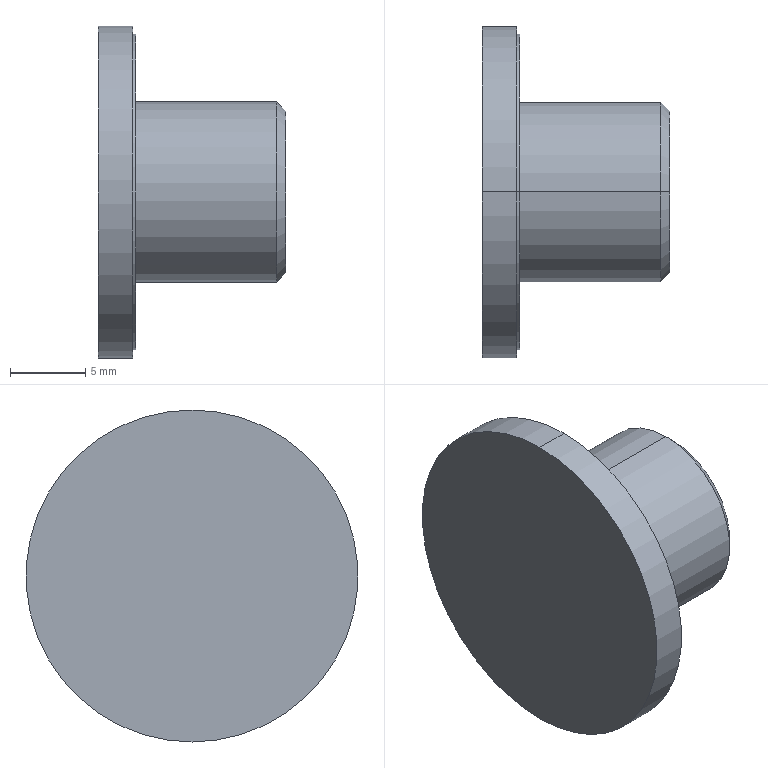Part | SolidWorks | features BaseBody 1 | 1 solid | 43 faces | box 12.5 x 22.1 x 22.1 mm | volume 1625 mm3 | cylinder 17 | plane 16 | cone 10 | commonest cylinder face diameters 1 x8 8.3 x2 12 x2 21 x2 22.1 x2 1.2 x1
STEP:
#1=CARTESIAN_POINT('',(49.5,0.,-11.05));
#2=VERTEX_POINT('',#1);
#3=CARTESIAN_POINT('',(49.5,0.,11.05));
#4=VERTEX_POINT('',#3);
#5=CARTESIAN_POINT('',(49.5,0.,0.));
#6=DIRECTION('',(1.,0.,0.));
#7=DIRECTION('',(0.,0.,-1.));
#8=AXIS2_PLACEMENT_3D('',#5,#6,#7);
#9=CIRCLE('',#8,11.05);
#10=EDGE_CURVE('',#2,#4,#9,.T.);
#11=ORIENTED_EDGE('',*,*,#10,.T.);
#12=CARTESIAN_POINT('',(51.8,0.,11.05));
#13=VERTEX_POINT('',#12);
#14=CARTESIAN_POINT('',(52.,0.,11.05));
#15=DIRECTION('',(1.,0.,0.));
#16=VECTOR('',#15,1000.);
#17=LINE('',#14,#16);
#18=EDGE_CURVE('',#4,#13,#17,.T.);
#19=ORIENTED_EDGE('',*,*,#18,.T.);
#20=CARTESIAN_POINT('',(51.8,0.,-11.05));
#21=VERTEX_POINT('',#20);
#22=CARTESIAN_POINT('',(51.8,0.,0.));
#23=DIRECTION('',(-1.,0.,0.));
#24=DIRECTION('',(0.,0.,-1.));
#25=AXIS2_PLACEMENT_3D('',#22,#23,#24);
#26=CIRCLE('',#25,11.05);
#27=EDGE_CURVE('',#13,#21,#26,.T.);
#28=ORIENTED_EDGE('',*,*,#27,.T.);
#29=CARTESIAN_POINT('',(52.,0.,-11.05));
#30=DIRECTION('',(1.,0.,0.));
#31=VECTOR('',#30,1000.);
#32=LINE('',#29,#31);
#33=EDGE_CURVE('',#2,#21,#32,.T.);
#34=ORIENTED_EDGE('',*,*,#33,.F.);
#35=EDGE_LOOP('',(#11,#19,#28,#34));
#36=FACE_OUTER_BOUND('',#35,.T.);
#37=CARTESIAN_POINT('',(52.,0.,0.));
#38=DIRECTION('',(1.,0.,0.));
#39=DIRECTION('',(0.,0.,-1.));
#40=AXIS2_PLACEMENT_3D('',#37,#38,#39);
#41=CYLINDRICAL_SURFACE('',#40,11.05);
#42=ADVANCED_FACE('',(#36),#41,.T.);
#43=CARTESIAN_POINT('',(51.8,0.,10.5));
#44=VERTEX_POINT('',#43);
#45=CARTESIAN_POINT('',(51.8,0.,-10.5));
#46=VERTEX_POINT('',#45);
#47=CARTESIAN_POINT('',(51.8,0.,0.));
#48=DIRECTION('',(-1.,0.,0.));
#49=DIRECTION('',(0.,0.,-1.));
#50=AXIS2_PLACEMENT_3D('',#47,#48,#49);
#51=CIRCLE('',#50,10.5);
#52=EDGE_CURVE('',#44,#46,#51,.T.);
#53=ORIENTED_EDGE('',*,*,#52,.F.);
#54=CARTESIAN_POINT('',(52.,0.,10.5));
#55=VERTEX_POINT('',#54);
#56=CARTESIAN_POINT('',(52.,0.,10.5));
#57=DIRECTION('',(1.,0.,0.));
#58=VECTOR('',#57,1000.);
#59=LINE('',#56,#58);
#60=EDGE_CURVE('',#44,#55,#59,.T.);
#61=ORIENTED_EDGE('',*,*,#60,.T.);
#62=CARTESIAN_POINT('',(52.,0.,-10.5));
#63=VERTEX_POINT('',#62);
#64=CARTESIAN_POINT('',(52.,0.,0.));
#65=DIRECTION('',(-1.,0.,0.));
#66=DIRECTION('',(0.,0.,-1.));
#67=AXIS2_PLACEMENT_3D('',#64,#65,#66);
#68=CIRCLE('',#67,10.5);
#69=EDGE_CURVE('',#55,#63,#68,.T.);
#70=ORIENTED_EDGE('',*,*,#69,.T.);
#71=CARTESIAN_POINT('',(52.,0.,-10.5));
#72=DIRECTION('',(1.,0.,0.));
#73=VECTOR('',#72,1000.);
#74=LINE('',#71,#73);
#75=EDGE_CURVE('',#46,#63,#74,.T.);
#76=ORIENTED_EDGE('',*,*,#75,.F.);
#77=EDGE_LOOP('',(#53,#61,#70,#76));
#78=FACE_OUTER_BOUND('',#77,.T.);
#79=CARTESIAN_POINT('',(52.,0.,0.));
#80=DIRECTION('',(1.,0.,0.));
#81=DIRECTION('',(0.,0.,-1.));
#82=AXIS2_PLACEMENT_3D('',#79,#80,#81);
#83=CYLINDRICAL_SURFACE('',#82,10.5);
#84=ADVANCED_FACE('',(#78),#83,.T.);
#85=CARTESIAN_POINT('',(52.,0.,6.));
#86=VERTEX_POINT('',#85);
#87=CARTESIAN_POINT('',(52.,0.,-6.));
#88=VERTEX_POINT('',#87);
#89=CARTESIAN_POINT('',(52.,0.,0.));
#90=DIRECTION('',(-1.,0.,0.));
#91=DIRECTION('',(0.,0.,-1.));
#92=AXIS2_PLACEMENT_3D('',#89,#90,#91);
#93=CIRCLE('',#92,6.);
#94=EDGE_CURVE('',#86,#88,#93,.T.);
#95=ORIENTED_EDGE('',*,*,#94,.F.);
#96=CARTESIAN_POINT('',(61.386,0.,6.));
#97=VERTEX_POINT('',#96);
#98=CARTESIAN_POINT('',(56.693,0.,6.));
#99=DIRECTION('',(1.,0.,0.));
#100=VECTOR('',#99,1000.);
#101=LINE('',#98,#100);
#102=EDGE_CURVE('',#86,#97,#101,.T.);
#103=ORIENTED_EDGE('',*,*,#102,.T.);
#104=CARTESIAN_POINT('',(61.386,0.,-6.));
#105=VERTEX_POINT('',#104);
#106=CARTESIAN_POINT('',(61.386,0.,0.));
#107=DIRECTION('',(-1.,0.,0.));
#108=DIRECTION('',(0.,0.,-1.));
#109=AXIS2_PLACEMENT_3D('',#106,#107,#108);
#110=CIRCLE('',#109,6.);
#111=EDGE_CURVE('',#97,#105,#110,.T.);
#112=ORIENTED_EDGE('',*,*,#111,.T.);
#113=CARTESIAN_POINT('',(56.693,0.,-6.));
#114=DIRECTION('',(1.,0.,0.));
#115=VECTOR('',#114,1000.);
#116=LINE('',#113,#115);
#117=EDGE_CURVE('',#88,#105,#116,.T.);
#118=ORIENTED_EDGE('',*,*,#117,.F.);
#119=EDGE_LOOP('',(#95,#103,#112,#118));
#120=FACE_OUTER_BOUND('',#119,.T.);
#121=CARTESIAN_POINT('',(56.693,0.,0.));
#122=DIRECTION('',(1.,0.,0.));
#123=DIRECTION('',(0.,0.,-1.));
#124=AXIS2_PLACEMENT_3D('',#121,#122,#123);
#125=CYLINDRICAL_SURFACE('',#124,6.);
#126=ADVANCED_FACE('',(#120),#125,.T.);
#127=CARTESIAN_POINT('',(62.,0.,5.387));
#128=VERTEX_POINT('',#127);
#129=CARTESIAN_POINT('',(62.,0.,-5.387));
#130=VERTEX_POINT('',#129);
#131=CARTESIAN_POINT('',(62.,0.,0.));
#132=DIRECTION('',(-1.,0.,0.));
#133=DIRECTION('',(0.,0.,1.));
#134=AXIS2_PLACEMENT_3D('',#131,#132,#133);
#135=CIRCLE('',#134,5.387);
#136=EDGE_CURVE('',#128,#130,#135,.T.);
#137=ORIENTED_EDGE('',*,*,#136,.T.);
#138=CARTESIAN_POINT('',(61.387,0.,-6.));
#139=DIRECTION('',(-0.7071,0.,-0.7071));
#140=VECTOR('',#139,1000.);
#141=LINE('',#138,#140);
#142=EDGE_CURVE('',#130,#105,#141,.T.);
#143=ORIENTED_EDGE('',*,*,#142,.T.);
#144=ORIENTED_EDGE('',*,*,#111,.F.);
#145=CARTESIAN_POINT('',(61.387,0.,6.));
#146=DIRECTION('',(-0.7071,0.,0.7071));
#147=VECTOR('',#146,1000.);
#148=LINE('',#145,#147);
#149=EDGE_CURVE('',#128,#97,#148,.T.);
#150=ORIENTED_EDGE('',*,*,#149,.F.);
#151=EDGE_LOOP('',(#137,#143,#144,#150));
#152=FACE_OUTER_BOUND('',#151,.T.);
#153=CARTESIAN_POINT('',(61.387,0.,0.));
#154=DIRECTION('',(-1.,0.,0.));
#155=DIRECTION('',(0.,0.,1.));
#156=AXIS2_PLACEMENT_3D('',#153,#154,#155);
#157=CONICAL_SURFACE('',#156,6.,0.7854);
#158=ADVANCED_FACE('',(#152),#157,.T.);
#159=CARTESIAN_POINT('',(53.1,0.,4.15));
#160=VERTEX_POINT('',#159);
#161=CARTESIAN_POINT('',(53.1,0.,-4.15));
#162=VERTEX_POINT('',#161);
#163=CARTESIAN_POINT('',(53.1,0.,0.));
#164=DIRECTION('',(1.,0.,0.));
#165=DIRECTION('',(0.,0.,-1.));
#166=AXIS2_PLACEMENT_3D('',#163,#164,#165);
#167=CIRCLE('',#166,4.15);
#168=EDGE_CURVE('',#160,#162,#167,.T.);
#169=ORIENTED_EDGE('',*,*,#168,.F.);
#170=CARTESIAN_POINT('',(62.,0.,4.15));
#171=VERTEX_POINT('',#170);
#172=CARTESIAN_POINT('',(57.55,0.,4.15));
#173=DIRECTION('',(1.,0.,0.));
#174=VECTOR('',#173,1000.);
#175=LINE('',#172,#174);
#176=EDGE_CURVE('',#160,#171,#175,.T.);
#177=ORIENTED_EDGE('',*,*,#176,.T.);
#178=CARTESIAN_POINT('',(62.,0.,-4.15));
#179=VERTEX_POINT('',#178);
#180=CARTESIAN_POINT('',(62.,0.,0.));
#181=DIRECTION('',(-1.,0.,0.));
#182=DIRECTION('',(0.,0.,-1.));
#183=AXIS2_PLACEMENT_3D('',#180,#181,#182);
#184=CIRCLE('',#183,4.15);
#185=EDGE_CURVE('',#179,#171,#184,.T.);
#186=ORIENTED_EDGE('',*,*,#185,.F.);
#187=CARTESIAN_POINT('',(57.55,0.,-4.15));
#188=DIRECTION('',(1.,0.,0.));
#189=VECTOR('',#188,1000.);
#190=LINE('',#187,#189);
#191=EDGE_CURVE('',#162,#179,#190,.T.);
#192=ORIENTED_EDGE('',*,*,#191,.F.);
#193=EDGE_LOOP('',(#169,#177,#186,#192));
#194=FACE_OUTER_BOUND('',#193,.T.);
#195=CARTESIAN_POINT('',(57.55,0.,0.));
#196=DIRECTION('',(1.,0.,0.));
#197=DIRECTION('',(0.,0.,-1.));
#198=AXIS2_PLACEMENT_3D('',#195,#196,#197);
#199=CYLINDRICAL_SURFACE('',#198,4.15);
#200=ADVANCED_FACE('',(#194),#199,.F.);
#201=CARTESIAN_POINT('',(53.1,0.,3.));
#202=VERTEX_POINT('',#201);
#203=CARTESIAN_POINT('',(53.1,0.,2.));
#204=VERTEX_POINT('',#203);
#205=CARTESIAN_POINT('',(53.1,0.,2.5));
#206=DIRECTION('',(-1.,0.,0.));
#207=DIRECTION('',(0.,0.,-1.));
#208=AXIS2_PLACEMENT_3D('',#205,#206,#207);
#209=CIRCLE('',#208,0.5);
#210=EDGE_CURVE('',#202,#204,#209,.T.);
#211=ORIENTED_EDGE('',*,*,#210,.F.);
#212=CARTESIAN_POINT('',(59.067,0.,3.));
#213=VERTEX_POINT('',#212);
#214=CARTESIAN_POINT('',(56.083,0.,3.));
#215=DIRECTION('',(1.,0.,0.));
#216=VECTOR('',#215,1000.);
#217=LINE('',#214,#216);
#218=EDGE_CURVE('',#202,#213,#217,.T.);
#219=ORIENTED_EDGE('',*,*,#218,.T.);
#220=CARTESIAN_POINT('',(59.067,0.5,2.5));
#221=VERTEX_POINT('',#220);
#222=CARTESIAN_POINT('',(59.067,0.,2.5));
#223=DIRECTION('',(-1.,0.,0.));
#224=DIRECTION('',(0.,0.,-1.));
#225=AXIS2_PLACEMENT_3D('',#222,#223,#224);
#226=CIRCLE('',#225,0.5);
#227=EDGE_CURVE('',#213,#221,#226,.T.);
#228=ORIENTED_EDGE('',*,*,#227,.T.);
#229=CARTESIAN_POINT('',(59.067,0.,2.));
#230=VERTEX_POINT('',#229);
#231=CARTESIAN_POINT('',(59.067,0.,2.5));
#232=DIRECTION('',(-1.,0.,0.));
#233=DIRECTION('',(0.,0.,-1.));
#234=AXIS2_PLACEMENT_3D('',#231,#232,#233);
#235=CIRCLE('',#234,0.5);
#236=EDGE_CURVE('',#221,#230,#235,.T.);
#237=ORIENTED_EDGE('',*,*,#236,.T.);
#238=CARTESIAN_POINT('',(56.083,0.,2.));
#239=DIRECTION('',(1.,0.,0.));
#240=VECTOR('',#239,1000.);
#241=LINE('',#238,#240);
#242=EDGE_CURVE('',#204,#230,#241,.T.);
#243=ORIENTED_EDGE('',*,*,#242,.F.);
#244=EDGE_LOOP('',(#211,#219,#228,#237,#243));
#245=FACE_OUTER_BOUND('',#244,.T.);
#246=CARTESIAN_POINT('',(56.083,0.,2.5));
#247=DIRECTION('',(1.,0.,0.));
#248=DIRECTION('',(0.,0.,-1.));
#249=AXIS2_PLACEMENT_3D('',#246,#247,#248);
#250=CYLINDRICAL_SURFACE('',#249,0.5);
#251=ADVANCED_FACE('',(#245),#250,.T.);
#252=CARTESIAN_POINT('',(53.1,-2.5,0.5));
#253=VERTEX_POINT('',#252);
#254=CARTESIAN_POINT('',(53.1,-2.5,-0.5));
#255=VERTEX_POINT('',#254);
#256=CARTESIAN_POINT('',(53.1,-2.5,0.));
#257=DIRECTION('',(-1.,0.,0.));
#258=DIRECTION('',(0.,0.,-1.));
#259=AXIS2_PLACEMENT_3D('',#256,#257,#258);
#260=CIRCLE('',#259,0.5);
#261=EDGE_CURVE('',#253,#255,#260,.T.);
#262=ORIENTED_EDGE('',*,*,#261,.F.);
#263=CARTESIAN_POINT('',(59.067,-2.5,0.5));
#264=VERTEX_POINT('',#263);
#265=CARTESIAN_POINT('',(56.083,-2.5,0.5));
#266=DIRECTION('',(1.,0.,0.));
#267=VECTOR('',#266,1000.);
#268=LINE('',#265,#267);
#269=EDGE_CURVE('',#253,#264,#268,.T.);
#270=ORIENTED_EDGE('',*,*,#269,.T.);
#271=CARTESIAN_POINT('',(59.067,-2.5,-0.5));
#272=VERTEX_POINT('',#271);
#273=CARTESIAN_POINT('',(59.067,-2.5,0.));
#274=DIRECTION('',(-1.,0.,0.));
#275=DIRECTION('',(0.,0.,-1.));
#276=AXIS2_PLACEMENT_3D('',#273,#274,#275);
#277=CIRCLE('',#276,0.5);
#278=EDGE_CURVE('',#264,#272,#277,.T.);
#279=ORIENTED_EDGE('',*,*,#278,.T.);
#280=CARTESIAN_POINT('',(56.083,-2.5,-0.5));
#281=DIRECTION('',(1.,0.,0.));
#282=VECTOR('',#281,1000.);
#283=LINE('',#280,#282);
#284=EDGE_CURVE('',#255,#272,#283,.T.);
#285=ORIENTED_EDGE('',*,*,#284,.F.);
#286=EDGE_LOOP('',(#262,#270,#279,#285));
#287=FACE_OUTER_BOUND('',#286,.T.);
#288=CARTESIAN_POINT('',(56.083,-2.5,0.));
#289=DIRECTION('',(1.,0.,0.));
#290=DIRECTION('',(0.,0.,-1.));
#291=AXIS2_PLACEMENT_3D('',#288,#289,#290);
#292=CYLINDRICAL_SURFACE('',#291,0.5);
#293=ADVANCED_FACE('',(#287),#292,.T.);
#294=CARTESIAN_POINT('',(53.1,0.,-2.));
#295=VERTEX_POINT('',#294);
#296=CARTESIAN_POINT('',(53.1,0.,-3.));
#297=VERTEX_POINT('',#296);
#298=CARTESIAN_POINT('',(53.1,0.,-2.5));
#299=DIRECTION('',(-1.,0.,0.));
#300=DIRECTION('',(0.,0.,-1.));
#301=AXIS2_PLACEMENT_3D('',#298,#299,#300);
#302=CIRCLE('',#301,0.5);
#303=EDGE_CURVE('',#295,#297,#302,.T.);
#304=ORIENTED_EDGE('',*,*,#303,.F.);
#305=CARTESIAN_POINT('',(59.067,0.,-2.));
#306=VERTEX_POINT('',#305);
#307=CARTESIAN_POINT('',(56.083,0.,-2.));
#308=DIRECTION('',(1.,0.,0.));
#309=VECTOR('',#308,1000.);
#310=LINE('',#307,#309);
#311=EDGE_CURVE('',#295,#306,#310,.T.);
#312=ORIENTED_EDGE('',*,*,#311,.T.);
#313=CARTESIAN_POINT('',(59.067,0.5,-2.5));
#314=VERTEX_POINT('',#313);
#315=CARTESIAN_POINT('',(59.067,0.,-2.5));
#316=DIRECTION('',(-1.,0.,0.));
#317=DIRECTION('',(0.,0.,-1.));
#318=AXIS2_PLACEMENT_3D('',#315,#316,#317);
#319=CIRCLE('',#318,0.5);
#320=EDGE_CURVE('',#306,#314,#319,.T.);
#321=ORIENTED_EDGE('',*,*,#320,.T.);
#322=CARTESIAN_POINT('',(59.067,0.,-3.));
#323=VERTEX_POINT('',#322);
#324=CARTESIAN_POINT('',(59.067,0.,-2.5));
#325=DIRECTION('',(-1.,0.,0.));
#326=DIRECTION('',(0.,0.,-1.));
#327=AXIS2_PLACEMENT_3D('',#324,#325,#326);
#328=CIRCLE('',#327,0.5);
#329=EDGE_CURVE('',#314,#323,#328,.T.);
#330=ORIENTED_EDGE('',*,*,#329,.T.);
#331=CARTESIAN_POINT('',(56.083,0.,-3.));
#332=DIRECTION('',(1.,0.,0.));
#333=VECTOR('',#332,1000.);
#334=LINE('',#331,#333);
#335=EDGE_CURVE('',#297,#323,#334,.T.);
#336=ORIENTED_EDGE('',*,*,#335,.F.);
#337=EDGE_LOOP('',(#304,#312,#321,#330,#336));
#338=FACE_OUTER_BOUND('',#337,.T.);
#339=CARTESIAN_POINT('',(56.083,0.,-2.5));
#340=DIRECTION('',(1.,0.,0.));
#341=DIRECTION('',(0.,0.,-1.));
#342=AXIS2_PLACEMENT_3D('',#339,#340,#341);
#343=CYLINDRICAL_SURFACE('',#342,0.5);
#344=ADVANCED_FACE('',(#338),#343,.T.);
#345=CARTESIAN_POINT('',(53.1,2.5,0.5));
#346=VERTEX_POINT('',#345);
#347=CARTESIAN_POINT('',(53.1,2.5,-0.5));
#348=VERTEX_POINT('',#347);
#349=CARTESIAN_POINT('',(53.1,2.5,0.));
#350=DIRECTION('',(-1.,0.,0.));
#351=DIRECTION('',(0.,0.,-1.));
#352=AXIS2_PLACEMENT_3D('',#349,#350,#351);
#353=CIRCLE('',#352,0.5);
#354=EDGE_CURVE('',#346,#348,#353,.T.);
#355=ORIENTED_EDGE('',*,*,#354,.F.);
#356=CARTESIAN_POINT('',(59.067,2.5,0.5));
#357=VERTEX_POINT('',#356);
#358=CARTESIAN_POINT('',(56.083,2.5,0.5));
#359=DIRECTION('',(1.,0.,0.));
#360=VECTOR('',#359,1000.);
#361=LINE('',#358,#360);
#362=EDGE_CURVE('',#346,#357,#361,.T.);
#363=ORIENTED_EDGE('',*,*,#362,.T.);
#364=CARTESIAN_POINT('',(59.067,2.5,-0.5));
#365=VERTEX_POINT('',#364);
#366=CARTESIAN_POINT('',(59.067,2.5,0.));
#367=DIRECTION('',(-1.,0.,0.));
#368=DIRECTION('',(0.,0.,-1.));
#369=AXIS2_PLACEMENT_3D('',#366,#367,#368);
#370=CIRCLE('',#369,0.5);
#371=EDGE_CURVE('',#357,#365,#370,.T.);
#372=ORIENTED_EDGE('',*,*,#371,.T.);
#373=CARTESIAN_POINT('',(56.083,2.5,-0.5));
#374=DIRECTION('',(1.,0.,0.));
#375=VECTOR('',#374,1000.);
#376=LINE('',#373,#375);
#377=EDGE_CURVE('',#348,#365,#376,.T.);
#378=ORIENTED_EDGE('',*,*,#377,.F.);
#379=EDGE_LOOP('',(#355,#363,#372,#378));
#380=FACE_OUTER_BOUND('',#379,.T.);
#381=CARTESIAN_POINT('',(56.083,2.5,0.));
#382=DIRECTION('',(1.,0.,0.));
#383=DIRECTION('',(0.,0.,-1.));
#384=AXIS2_PLACEMENT_3D('',#381,#382,#383);
#385=CYLINDRICAL_SURFACE('',#384,0.5);
#386=ADVANCED_FACE('',(#380),#385,.T.);
#387=CARTESIAN_POINT('',(60.,-0.25,2.5));
#388=VERTEX_POINT('',#387);
#389=CARTESIAN_POINT('',(60.,0.25,2.5));
#390=VERTEX_POINT('',#389);
#391=CARTESIAN_POINT('',(60.,0.,2.5));
#392=DIRECTION('',(-1.,0.,0.));
#393=DIRECTION('',(0.,-1.,0.));
#394=AXIS2_PLACEMENT_3D('',#391,#392,#393);
#395=CIRCLE('',#394,0.25);
#396=EDGE_CURVE('',#388,#390,#395,.T.);
#397=ORIENTED_EDGE('',*,*,#396,.T.);
#398=CARTESIAN_POINT('',(59.067,0.5,2.5));
#399=DIRECTION('',(-0.9659,0.2588,0.));
#400=VECTOR('',#399,1000.);
#401=LINE('',#398,#400);
#402=EDGE_CURVE('',#390,#221,#401,.T.);
#403=ORIENTED_EDGE('',*,*,#402,.T.);
#404=ORIENTED_EDGE('',*,*,#227,.F.);
#405=CARTESIAN_POINT('',(59.067,-0.5,2.5));
#406=VERTEX_POINT('',#405);
#407=CARTESIAN_POINT('',(59.067,0.,2.5));
#408=DIRECTION('',(-1.,0.,0.));
#409=DIRECTION('',(0.,0.,-1.));
#410=AXIS2_PLACEMENT_3D('',#407,#408,#409);
#411=CIRCLE('',#410,0.5);
#412=EDGE_CURVE('',#406,#213,#411,.T.);
#413=ORIENTED_EDGE('',*,*,#412,.F.);
#414=CARTESIAN_POINT('',(59.067,-0.5,2.5));
#415=DIRECTION('',(-0.9659,-0.2588,0.));
#416=VECTOR('',#415,1000.);
#417=LINE('',#414,#416);
#418=EDGE_CURVE('',#388,#406,#417,.T.);
#419=ORIENTED_EDGE('',*,*,#418,.F.);
#420=EDGE_LOOP('',(#397,#403,#404,#413,#419));
#421=FACE_OUTER_BOUND('',#420,.T.);
#422=CARTESIAN_POINT('',(59.067,0.,2.5));
#423=DIRECTION('',(-1.,0.,0.));
#424=DIRECTION('',(0.,-1.,0.));
#425=AXIS2_PLACEMENT_3D('',#422,#423,#424);
#426=CONICAL_SURFACE('',#425,0.5,0.2618);
#427=ADVANCED_FACE('',(#421),#426,.T.);
#428=CARTESIAN_POINT('',(60.,-2.5,0.25));
#429=VERTEX_POINT('',#428);
#430=CARTESIAN_POINT('',(60.,-2.5,-0.25));
#431=VERTEX_POINT('',#430);
#432=CARTESIAN_POINT('',(60.,-2.5,0.));
#433=DIRECTION('',(-1.,0.,0.));
#434=DIRECTION('',(0.,0.,1.));
#435=AXIS2_PLACEMENT_3D('',#432,#433,#434);
#436=CIRCLE('',#435,0.25);
#437=EDGE_CURVE('',#429,#431,#436,.T.);
#438=ORIENTED_EDGE('',*,*,#437,.T.);
#439=CARTESIAN_POINT('',(59.067,-2.5,-0.5));
#440=DIRECTION('',(-0.9659,0.,-0.2588));
#441=VECTOR('',#440,1000.);
#442=LINE('',#439,#441);
#443=EDGE_CURVE('',#431,#272,#442,.T.);
#444=ORIENTED_EDGE('',*,*,#443,.T.);
#445=ORIENTED_EDGE('',*,*,#278,.F.);
#446=CARTESIAN_POINT('',(59.067,-2.5,0.5));
#447=DIRECTION('',(-0.9659,0.,0.2588));
#448=VECTOR('',#447,1000.);
#449=LINE('',#446,#448);
#450=EDGE_CURVE('',#429,#264,#449,.T.);
#451=ORIENTED_EDGE('',*,*,#450,.F.);
#452=EDGE_LOOP('',(#438,#444,#445,#451));
#453=FACE_OUTER_BOUND('',#452,.T.);
#454=CARTESIAN_POINT('',(59.067,-2.5,0.));
#455=DIRECTION('',(-1.,0.,0.));
#456=DIRECTION('',(0.,0.,1.));
#457=AXIS2_PLACEMENT_3D('',#454,#455,#456);
#458=CONICAL_SURFACE('',#457,0.5,0.2618);
#459=ADVANCED_FACE('',(#453),#458,.T.);
#460=CARTESIAN_POINT('',(60.,-0.25,-2.5));
#461=VERTEX_POINT('',#460);
#462=CARTESIAN_POINT('',(60.,0.25,-2.5));
#463=VERTEX_POINT('',#462);
#464=CARTESIAN_POINT('',(60.,0.,-2.5));
#465=DIRECTION('',(-1.,0.,0.));
#466=DIRECTION('',(0.,-1.,0.));
#467=AXIS2_PLACEMENT_3D('',#464,#465,#466);
#468=CIRCLE('',#467,0.25);
#469=EDGE_CURVE('',#461,#463,#468,.T.);
#470=ORIENTED_EDGE('',*,*,#469,.T.);
#471=CARTESIAN_POINT('',(59.067,0.5,-2.5));
#472=DIRECTION('',(-0.9659,0.2588,0.));
#473=VECTOR('',#472,1000.);
#474=LINE('',#471,#473);
#475=EDGE_CURVE('',#463,#314,#474,.T.);
#476=ORIENTED_EDGE('',*,*,#475,.T.);
#477=ORIENTED_EDGE('',*,*,#320,.F.);
#478=CARTESIAN_POINT('',(59.067,-0.5,-2.5));
#479=VERTEX_POINT('',#478);
#480=CARTESIAN_POINT('',(59.067,0.,-2.5));
#481=DIRECTION('',(-1.,0.,0.));
#482=DIRECTION('',(0.,0.,-1.));
#483=AXIS2_PLACEMENT_3D('',#480,#481,#482);
#484=CIRCLE('',#483,0.5);
#485=EDGE_CURVE('',#479,#306,#484,.T.);
#486=ORIENTED_EDGE('',*,*,#485,.F.);
#487=CARTESIAN_POINT('',(59.067,-0.5,-2.5));
#488=DIRECTION('',(-0.9659,-0.2588,0.));
#489=VECTOR('',#488,1000.);
#490=LINE('',#487,#489);
#491=EDGE_CURVE('',#461,#479,#490,.T.);
#492=ORIENTED_EDGE('',*,*,#491,.F.);
#493=EDGE_LOOP('',(#470,#476,#477,#486,#492));
#494=FACE_OUTER_BOUND('',#493,.T.);
#495=CARTESIAN_POINT('',(59.067,0.,-2.5));
#496=DIRECTION('',(-1.,0.,0.));
#497=DIRECTION('',(0.,-1.,0.));
#498=AXIS2_PLACEMENT_3D('',#495,#496,#497);
#499=CONICAL_SURFACE('',#498,0.5,0.2618);
#500=ADVANCED_FACE('',(#494),#499,.T.);
#501=CARTESIAN_POINT('',(60.,2.5,0.25));
#502=VERTEX_POINT('',#501);
#503=CARTESIAN_POINT('',(60.,2.5,-0.25));
#504=VERTEX_POINT('',#503);
#505=CARTESIAN_POINT('',(60.,2.5,0.));
#506=DIRECTION('',(-1.,0.,0.));
#507=DIRECTION('',(0.,0.,1.));
#508=AXIS2_PLACEMENT_3D('',#505,#506,#507);
#509=CIRCLE('',#508,0.25);
#510=EDGE_CURVE('',#502,#504,#509,.T.);
#511=ORIENTED_EDGE('',*,*,#510,.T.);
#512=CARTESIAN_POINT('',(59.067,2.5,-0.5));
#513=DIRECTION('',(-0.9659,0.,-0.2588));
#514=VECTOR('',#513,1000.);
#515=LINE('',#512,#514);
#516=EDGE_CURVE('',#504,#365,#515,.T.);
#517=ORIENTED_EDGE('',*,*,#516,.T.);
#518=ORIENTED_EDGE('',*,*,#371,.F.);
#519=CARTESIAN_POINT('',(59.067,2.5,0.5));
#520=DIRECTION('',(-0.9659,0.,0.2588));
#521=VECTOR('',#520,1000.);
#522=LINE('',#519,#521);
#523=EDGE_CURVE('',#502,#357,#522,.T.);
#524=ORIENTED_EDGE('',*,*,#523,.F.);
#525=EDGE_LOOP('',(#511,#517,#518,#524));
#526=FACE_OUTER_BOUND('',#525,.T.);
#527=CARTESIAN_POINT('',(59.067,2.5,0.));
#528=DIRECTION('',(-1.,0.,0.));
#529=DIRECTION('',(0.,0.,1.));
#530=AXIS2_PLACEMENT_3D('',#527,#528,#529);
#531=CONICAL_SURFACE('',#530,0.5,0.2618);
#532=ADVANCED_FACE('',(#526),#531,.T.);
#533=ORIENTED_EDGE('',*,*,#10,.F.);
#534=CARTESIAN_POINT('',(49.5,0.,0.));
#535=DIRECTION('',(1.,0.,0.));
#536=DIRECTION('',(0.,0.,-1.));
#537=AXIS2_PLACEMENT_3D('',#534,#535,#536);
#538=CIRCLE('',#537,11.05);
#539=EDGE_CURVE('',#4,#2,#538,.T.);
#540=ORIENTED_EDGE('',*,*,#539,.F.);
#541=EDGE_LOOP('',(#533,#540));
#542=FACE_OUTER_BOUND('',#541,.T.);
#543=CARTESIAN_POINT('',(49.5,0.,0.));
#544=DIRECTION('',(1.,0.,0.));
#545=DIRECTION('',(0.,0.,-1.));
#546=AXIS2_PLACEMENT_3D('',#543,#544,#545);
#547=PLANE('',#546);
#548=ADVANCED_FACE('',(#542),#547,.F.);
#549=ORIENTED_EDGE('',*,*,#18,.F.);
#550=ORIENTED_EDGE('',*,*,#539,.T.);
#551=ORIENTED_EDGE('',*,*,#33,.T.);
#552=CARTESIAN_POINT('',(51.8,0.,0.));
#553=DIRECTION('',(-1.,0.,0.));
#554=DIRECTION('',(0.,0.,-1.));
#555=AXIS2_PLACEMENT_3D('',#552,#553,#554);
#556=CIRCLE('',#555,11.05);
#557=EDGE_CURVE('',#21,#13,#556,.T.);
#558=ORIENTED_EDGE('',*,*,#557,.T.);
#559=EDGE_LOOP('',(#549,#550,#551,#558));
#560=FACE_OUTER_BOUND('',#559,.T.);
#561=CARTESIAN_POINT('',(52.,0.,0.));
#562=DIRECTION('',(1.,0.,0.));
#563=DIRECTION('',(0.,0.,-1.));
#564=AXIS2_PLACEMENT_3D('',#561,#562,#563);
#565=CYLINDRICAL_SURFACE('',#564,11.05);
#566=ADVANCED_FACE('',(#560),#565,.T.);
#567=CARTESIAN_POINT('',(51.8,0.,0.));
#568=DIRECTION('',(-1.,0.,0.));
#569=DIRECTION('',(0.,0.,-1.));
#570=AXIS2_PLACEMENT_3D('',#567,#568,#569);
#571=CIRCLE('',#570,10.5);
#572=EDGE_CURVE('',#46,#44,#571,.T.);
#573=ORIENTED_EDGE('',*,*,#572,.T.);
#574=ORIENTED_EDGE('',*,*,#52,.T.);
#575=EDGE_LOOP('',(#573,#574));
#576=FACE_BOUND('',#575,.T.);
#577=ORIENTED_EDGE('',*,*,#557,.F.);
#578=ORIENTED_EDGE('',*,*,#27,.F.);
#579=EDGE_LOOP('',(#577,#578));
#580=FACE_OUTER_BOUND('',#579,.T.);
#581=CARTESIAN_POINT('',(51.8,0.,0.));
#582=DIRECTION('',(1.,0.,0.));
#583=DIRECTION('',(0.,0.,-1.));
#584=AXIS2_PLACEMENT_3D('',#581,#582,#583);
#585=PLANE('',#584);
#586=ADVANCED_FACE('',(#576,#580),#585,.T.);
#587=ORIENTED_EDGE('',*,*,#60,.F.);
#588=ORIENTED_EDGE('',*,*,#572,.F.);
#589=ORIENTED_EDGE('',*,*,#75,.T.);
#590=CARTESIAN_POINT('',(52.,0.,0.));
#591=DIRECTION('',(-1.,0.,0.));
#592=DIRECTION('',(0.,0.,-1.));
#593=AXIS2_PLACEMENT_3D('',#590,#591,#592);
#594=CIRCLE('',#593,10.5);
#595=EDGE_CURVE('',#63,#55,#594,.T.);
#596=ORIENTED_EDGE('',*,*,#595,.T.);
#597=EDGE_LOOP('',(#587,#588,#589,#596));
#598=FACE_OUTER_BOUND('',#597,.T.);
#599=CARTESIAN_POINT('',(52.,0.,0.));
#600=DIRECTION('',(1.,0.,0.));
#601=DIRECTION('',(0.,0.,-1.));
#602=AXIS2_PLACEMENT_3D('',#599,#600,#601);
#603=CYLINDRICAL_SURFACE('',#602,10.5);
#604=ADVANCED_FACE('',(#598),#603,.T.);
#605=CARTESIAN_POINT('',(52.,0.,0.));
#606=DIRECTION('',(-1.,0.,0.));
#607=DIRECTION('',(0.,0.,-1.));
#608=AXIS2_PLACEMENT_3D('',#605,#606,#607);
#609=CIRCLE('',#608,6.);
#610=EDGE_CURVE('',#88,#86,#609,.T.);
#611=ORIENTED_EDGE('',*,*,#610,.T.);
#612=ORIENTED_EDGE('',*,*,#94,.T.);
#613=EDGE_LOOP('',(#611,#612));
#614=FACE_BOUND('',#613,.T.);
#615=CARTESIAN_POINT('',(52.,6.35,0.7));
#616=VERTEX_POINT('',#615);
#617=CARTESIAN_POINT('',(52.,10.,0.));
#618=VERTEX_POINT('',#617);
#619=CARTESIAN_POINT('',(52.,6.35,0.7));
#620=DIRECTION('',(0.,0.9821,-0.1883));
#621=VECTOR('',#620,1000.);
#622=LINE('',#619,#621);
#623=EDGE_CURVE('',#616,#618,#622,.T.);
#624=ORIENTED_EDGE('',*,*,#623,.T.);
#625=CARTESIAN_POINT('',(52.,6.35,-0.7));
#626=VERTEX_POINT('',#625);
#627=CARTESIAN_POINT('',(52.,10.,0.));
#628=DIRECTION('',(0.,-0.9821,-0.1883));
#629=VECTOR('',#628,1000.);
#630=LINE('',#627,#629);
#631=EDGE_CURVE('',#618,#626,#630,.T.);
#632=ORIENTED_EDGE('',*,*,#631,.T.);
#633=CARTESIAN_POINT('',(52.,6.35,0.));
#634=DIRECTION('',(0.,0.,1.));
#635=VECTOR('',#634,1000.);
#636=LINE('',#633,#635);
#637=EDGE_CURVE('',#626,#616,#636,.T.);
#638=ORIENTED_EDGE('',*,*,#637,.T.);
#639=EDGE_LOOP('',(#624,#632,#638));
#640=FACE_BOUND('',#639,.T.);
#641=ORIENTED_EDGE('',*,*,#595,.F.);
#642=ORIENTED_EDGE('',*,*,#69,.F.);
#643=EDGE_LOOP('',(#641,#642));
#644=FACE_OUTER_BOUND('',#643,.T.);
#645=CARTESIAN_POINT('',(52.,0.,0.));
#646=DIRECTION('',(1.,0.,0.));
#647=DIRECTION('',(0.,0.,-1.));
#648=AXIS2_PLACEMENT_3D('',#645,#646,#647);
#649=PLANE('',#648);
#650=ADVANCED_FACE('',(#614,#640,#644),#649,.T.);
#651=ORIENTED_EDGE('',*,*,#102,.F.);
#652=ORIENTED_EDGE('',*,*,#610,.F.);
#653=ORIENTED_EDGE('',*,*,#117,.T.);
#654=CARTESIAN_POINT('',(61.386,0.,0.));
#655=DIRECTION('',(-1.,0.,0.));
#656=DIRECTION('',(0.,0.,-1.));
#657=AXIS2_PLACEMENT_3D('',#654,#655,#656);
#658=CIRCLE('',#657,6.);
#659=EDGE_CURVE('',#105,#97,#658,.T.);
#660=ORIENTED_EDGE('',*,*,#659,.T.);
#661=EDGE_LOOP('',(#651,#652,#653,#660));
#662=FACE_OUTER_BOUND('',#661,.T.);
#663=CARTESIAN_POINT('',(56.693,0.,0.));
#664=DIRECTION('',(1.,0.,0.));
#665=DIRECTION('',(0.,0.,-1.));
#666=AXIS2_PLACEMENT_3D('',#663,#664,#665);
#667=CYLINDRICAL_SURFACE('',#666,6.);
#668=ADVANCED_FACE('',(#662),#667,.T.);
#669=ORIENTED_EDGE('',*,*,#631,.F.);
#670=CARTESIAN_POINT('',(51.8,10.,0.));
#671=VERTEX_POINT('',#670);
#672=CARTESIAN_POINT('',(52.,10.,0.));
#673=DIRECTION('',(1.,0.,0.));
#674=VECTOR('',#673,1000.);
#675=LINE('',#672,#674);
#676=EDGE_CURVE('',#671,#618,#675,.T.);
#677=ORIENTED_EDGE('',*,*,#676,.F.);
#678=CARTESIAN_POINT('',(51.8,6.35,-0.7));
#679=VERTEX_POINT('',#678);
#680=CARTESIAN_POINT('',(51.8,6.35,-0.7));
#681=DIRECTION('',(0.,0.9821,0.1883));
#682=VECTOR('',#681,1000.);
#683=LINE('',#680,#682);
#684=EDGE_CURVE('',#679,#671,#683,.T.);
#685=ORIENTED_EDGE('',*,*,#684,.F.);
#686=CARTESIAN_POINT('',(52.,6.35,-0.7));
#687=DIRECTION('',(-1.,0.,0.));
#688=VECTOR('',#687,1000.);
#689=LINE('',#686,#688);
#690=EDGE_CURVE('',#626,#679,#689,.T.);
#691=ORIENTED_EDGE('',*,*,#690,.F.);
#692=EDGE_LOOP('',(#669,#677,#685,#691));
#693=FACE_OUTER_BOUND('',#692,.T.);
#694=CARTESIAN_POINT('',(52.,6.35,-0.7));
#695=DIRECTION('',(0.,0.1883,-0.9821));
#696=DIRECTION('',(0.,0.9821,0.1883));
#697=AXIS2_PLACEMENT_3D('',#694,#695,#696);
#698=PLANE('',#697);
#699=ADVANCED_FACE('',(#693),#698,.F.);
#700=ORIENTED_EDGE('',*,*,#623,.F.);
#701=CARTESIAN_POINT('',(51.8,6.35,0.7));
#702=VERTEX_POINT('',#701);
#703=CARTESIAN_POINT('',(52.,6.35,0.7));
#704=DIRECTION('',(1.,0.,0.));
#705=VECTOR('',#704,1000.);
#706=LINE('',#703,#705);
#707=EDGE_CURVE('',#702,#616,#706,.T.);
#708=ORIENTED_EDGE('',*,*,#707,.F.);
#709=CARTESIAN_POINT('',(51.8,10.,0.));
#710=DIRECTION('',(0.,-0.9821,0.1883));
#711=VECTOR('',#710,1000.);
#712=LINE('',#709,#711);
#713=EDGE_CURVE('',#671,#702,#712,.T.);
#714=ORIENTED_EDGE('',*,*,#713,.F.);
#715=ORIENTED_EDGE('',*,*,#676,.T.);
#716=EDGE_LOOP('',(#700,#708,#714,#715));
#717=FACE_OUTER_BOUND('',#716,.T.);
#718=CARTESIAN_POINT('',(52.,10.,0.));
#719=DIRECTION('',(0.,0.1883,0.9821));
#720=DIRECTION('',(0.,-0.9821,0.1883));
#721=AXIS2_PLACEMENT_3D('',#718,#719,#720);
#722=PLANE('',#721);
#723=ADVANCED_FACE('',(#717),#722,.F.);
#724=ORIENTED_EDGE('',*,*,#637,.F.);
#725=ORIENTED_EDGE('',*,*,#690,.T.);
#726=CARTESIAN_POINT('',(51.8,6.35,0.7));
#727=DIRECTION('',(0.,0.,-1.));
#728=VECTOR('',#727,1000.);
#729=LINE('',#726,#728);
#730=EDGE_CURVE('',#702,#679,#729,.T.);
#731=ORIENTED_EDGE('',*,*,#730,.F.);
#732=ORIENTED_EDGE('',*,*,#707,.T.);
#733=EDGE_LOOP('',(#724,#725,#731,#732));
#734=FACE_OUTER_BOUND('',#733,.T.);
#735=CARTESIAN_POINT('',(52.,6.35,0.7));
#736=DIRECTION('',(0.,-1.,0.));
#737=DIRECTION('',(0.,0.,-1.));
#738=AXIS2_PLACEMENT_3D('',#735,#736,#737);
#739=PLANE('',#738);
#740=ADVANCED_FACE('',(#734),#739,.F.);
#741=ORIENTED_EDGE('',*,*,#142,.F.);
#742=CARTESIAN_POINT('',(62.,0.,0.));
#743=DIRECTION('',(-1.,0.,0.));
#744=DIRECTION('',(0.,0.,1.));
#745=AXIS2_PLACEMENT_3D('',#742,#743,#744);
#746=CIRCLE('',#745,5.387);
#747=EDGE_CURVE('',#130,#128,#746,.T.);
#748=ORIENTED_EDGE('',*,*,#747,.T.);
#749=ORIENTED_EDGE('',*,*,#149,.T.);
#750=ORIENTED_EDGE('',*,*,#659,.F.);
#751=EDGE_LOOP('',(#741,#748,#749,#750));
#752=FACE_OUTER_BOUND('',#751,.T.);
#753=CARTESIAN_POINT('',(61.387,0.,0.));
#754=DIRECTION('',(-1.,0.,0.));
#755=DIRECTION('',(0.,0.,1.));
#756=AXIS2_PLACEMENT_3D('',#753,#754,#755);
#757=CONICAL_SURFACE('',#756,6.,0.7854);
#758=ADVANCED_FACE('',(#752),#757,.T.);
#759=ORIENTED_EDGE('',*,*,#730,.T.);
#760=ORIENTED_EDGE('',*,*,#684,.T.);
#761=ORIENTED_EDGE('',*,*,#713,.T.);
#762=EDGE_LOOP('',(#759,#760,#761));
#763=FACE_OUTER_BOUND('',#762,.T.);
#764=CARTESIAN_POINT('',(51.8,0.,0.));
#765=DIRECTION('',(1.,0.,0.));
#766=DIRECTION('',(0.,0.,-1.));
#767=AXIS2_PLACEMENT_3D('',#764,#765,#766);
#768=PLANE('',#767);
#769=ADVANCED_FACE('',(#763),#768,.T.);
#770=ORIENTED_EDGE('',*,*,#185,.T.);
#771=CARTESIAN_POINT('',(62.,0.,0.));
#772=DIRECTION('',(-1.,0.,0.));
#773=DIRECTION('',(0.,0.,-1.));
#774=AXIS2_PLACEMENT_3D('',#771,#772,#773);
#775=CIRCLE('',#774,4.15);
#776=EDGE_CURVE('',#171,#179,#775,.T.);
#777=ORIENTED_EDGE('',*,*,#776,.T.);
#778=EDGE_LOOP('',(#770,#777));
#779=FACE_BOUND('',#778,.T.);
#780=ORIENTED_EDGE('',*,*,#136,.F.);
#781=ORIENTED_EDGE('',*,*,#747,.F.);
#782=EDGE_LOOP('',(#780,#781));
#783=FACE_OUTER_BOUND('',#782,.T.);
#784=CARTESIAN_POINT('',(62.,4.768,0.));
#785=DIRECTION('',(1.,0.,0.));
#786=DIRECTION('',(0.,0.,-1.));
#787=AXIS2_PLACEMENT_3D('',#784,#785,#786);
#788=PLANE('',#787);
#789=ADVANCED_FACE('',(#779,#783),#788,.T.);
#790=ORIENTED_EDGE('',*,*,#176,.F.);
#791=CARTESIAN_POINT('',(53.1,3.328,-2.479));
#792=VERTEX_POINT('',#791);
#793=CARTESIAN_POINT('',(53.1,0.,0.));
#794=DIRECTION('',(1.,0.,0.));
#795=DIRECTION('',(0.,0.,-1.));
#796=AXIS2_PLACEMENT_3D('',#793,#794,#795);
#797=CIRCLE('',#796,4.15);
#798=EDGE_CURVE('',#792,#160,#797,.T.);
#799=ORIENTED_EDGE('',*,*,#798,.F.);
#800=CARTESIAN_POINT('',(61.5,3.328,-2.479));
#801=VERTEX_POINT('',#800);
#802=CARTESIAN_POINT('',(57.55,3.328,-2.479));
#803=DIRECTION('',(-1.,0.,0.));
#804=VECTOR('',#803,1000.);
#805=LINE('',#802,#804);
#806=EDGE_CURVE('',#801,#792,#805,.T.);
#807=ORIENTED_EDGE('',*,*,#806,.F.);
#808=CARTESIAN_POINT('',(61.5,2.479,-3.328));
#809=VERTEX_POINT('',#808);
#810=CARTESIAN_POINT('',(61.5,0.,0.));
#811=DIRECTION('',(1.,0.,0.));
#812=DIRECTION('',(0.,0.,-1.));
#813=AXIS2_PLACEMENT_3D('',#810,#811,#812);
#814=CIRCLE('',#813,4.15);
#815=EDGE_CURVE('',#809,#801,#814,.T.);
#816=ORIENTED_EDGE('',*,*,#815,.F.);
#817=CARTESIAN_POINT('',(53.1,2.479,-3.328));
#818=VERTEX_POINT('',#817);
#819=CARTESIAN_POINT('',(57.55,2.479,-3.328));
#820=DIRECTION('',(1.,0.,0.));
#821=VECTOR('',#820,1000.);
#822=LINE('',#819,#821);
#823=EDGE_CURVE('',#818,#809,#822,.T.);
#824=ORIENTED_EDGE('',*,*,#823,.F.);
#825=CARTESIAN_POINT('',(53.1,0.,0.));
#826=DIRECTION('',(1.,0.,0.));
#827=DIRECTION('',(0.,0.,-1.));
#828=AXIS2_PLACEMENT_3D('',#825,#826,#827);
#829=CIRCLE('',#828,4.15);
#830=EDGE_CURVE('',#162,#818,#829,.T.);
#831=ORIENTED_EDGE('',*,*,#830,.F.);
#832=ORIENTED_EDGE('',*,*,#191,.T.);
#833=ORIENTED_EDGE('',*,*,#776,.F.);
#834=EDGE_LOOP('',(#790,#799,#807,#816,#824,#831,#832,#833));
#835=FACE_OUTER_BOUND('',#834,.T.);
#836=CARTESIAN_POINT('',(57.55,0.,0.));
#837=DIRECTION('',(1.,0.,0.));
#838=DIRECTION('',(0.,0.,-1.));
#839=AXIS2_PLACEMENT_3D('',#836,#837,#838);
#840=CYLINDRICAL_SURFACE('',#839,4.15);
#841=ADVANCED_FACE('',(#835),#840,.F.);
#842=CARTESIAN_POINT('',(53.1,0.,2.5));
#843=DIRECTION('',(-1.,0.,0.));
#844=DIRECTION('',(0.,0.,-1.));
#845=AXIS2_PLACEMENT_3D('',#842,#843,#844);
#846=CIRCLE('',#845,0.5);
#847=EDGE_CURVE('',#204,#202,#846,.T.);
#848=ORIENTED_EDGE('',*,*,#847,.T.);
#849=ORIENTED_EDGE('',*,*,#210,.T.);
#850=EDGE_LOOP('',(#848,#849));
#851=FACE_BOUND('',#850,.T.);
#852=CARTESIAN_POINT('',(53.1,-2.5,0.));
#853=DIRECTION('',(-1.,0.,0.));
#854=DIRECTION('',(0.,0.,-1.));
#855=AXIS2_PLACEMENT_3D('',#852,#853,#854);
#856=CIRCLE('',#855,0.5);
#857=EDGE_CURVE('',#255,#253,#856,.T.);
#858=ORIENTED_EDGE('',*,*,#857,.T.);
#859=ORIENTED_EDGE('',*,*,#261,.T.);
#860=EDGE_LOOP('',(#858,#859));
#861=FACE_BOUND('',#860,.T.);
#862=CARTESIAN_POINT('',(53.1,0.,-2.5));
#863=DIRECTION('',(-1.,0.,0.));
#864=DIRECTION('',(0.,0.,-1.));
#865=AXIS2_PLACEMENT_3D('',#862,#863,#864);
#866=CIRCLE('',#865,0.5);
#867=EDGE_CURVE('',#297,#295,#866,.T.);
#868=ORIENTED_EDGE('',*,*,#867,.T.);
#869=ORIENTED_EDGE('',*,*,#303,.T.);
#870=EDGE_LOOP('',(#868,#869));
#871=FACE_BOUND('',#870,.T.);
#872=CARTESIAN_POINT('',(53.1,2.5,0.));
#873=DIRECTION('',(-1.,0.,0.));
#874=DIRECTION('',(0.,0.,-1.));
#875=AXIS2_PLACEMENT_3D('',#872,#873,#874);
#876=CIRCLE('',#875,0.5);
#877=EDGE_CURVE('',#348,#346,#876,.T.);
#878=ORIENTED_EDGE('',*,*,#877,.T.);
#879=ORIENTED_EDGE('',*,*,#354,.T.);
#880=EDGE_LOOP('',(#878,#879));
#881=FACE_BOUND('',#880,.T.);
#882=ORIENTED_EDGE('',*,*,#798,.T.);
#883=ORIENTED_EDGE('',*,*,#168,.T.);
#884=ORIENTED_EDGE('',*,*,#830,.T.);
#885=CARTESIAN_POINT('',(53.1,2.086,-2.934));
#886=VERTEX_POINT('',#885);
#887=CARTESIAN_POINT('',(53.1,2.479,-3.328));
#888=DIRECTION('',(0.,-0.7071,0.7071));
#889=VECTOR('',#888,1000.);
#890=LINE('',#887,#889);
#891=EDGE_CURVE('',#818,#886,#890,.T.);
#892=ORIENTED_EDGE('',*,*,#891,.T.);
#893=CARTESIAN_POINT('',(53.1,2.934,-2.086));
#894=VERTEX_POINT('',#893);
#895=CARTESIAN_POINT('',(53.1,2.51,-2.51));
#896=DIRECTION('',(-1.,0.,0.));
#897=DIRECTION('',(0.,0.,-1.));
#898=AXIS2_PLACEMENT_3D('',#895,#896,#897);
#899=CIRCLE('',#898,0.6);
#900=EDGE_CURVE('',#886,#894,#899,.T.);
#901=ORIENTED_EDGE('',*,*,#900,.T.);
#902=CARTESIAN_POINT('',(53.1,2.934,-2.086));
#903=DIRECTION('',(0.,0.7071,-0.7071));
#904=VECTOR('',#903,1000.);
#905=LINE('',#902,#904);
#906=EDGE_CURVE('',#894,#792,#905,.T.);
#907=ORIENTED_EDGE('',*,*,#906,.T.);
#908=EDGE_LOOP('',(#882,#883,#884,#892,#901,#907));
#909=FACE_OUTER_BOUND('',#908,.T.);
#910=CARTESIAN_POINT('',(53.1,2.075,0.));
#911=DIRECTION('',(1.,0.,0.));
#912=DIRECTION('',(0.,0.,-1.));
#913=AXIS2_PLACEMENT_3D('',#910,#911,#912);
#914=PLANE('',#913);
#915=ADVANCED_FACE('',(#851,#861,#871,#881,#909),#914,.T.);
#916=CARTESIAN_POINT('',(61.5,2.934,-2.086));
#917=VERTEX_POINT('',#916);
#918=CARTESIAN_POINT('',(61.5,3.328,-2.479));
#919=DIRECTION('',(0.,-0.7071,0.7071));
#920=VECTOR('',#919,1000.);
#921=LINE('',#918,#920);
#922=EDGE_CURVE('',#801,#917,#921,.T.);
#923=ORIENTED_EDGE('',*,*,#922,.F.);
#924=ORIENTED_EDGE('',*,*,#806,.T.);
#925=ORIENTED_EDGE('',*,*,#906,.F.);
#926=CARTESIAN_POINT('',(61.5,2.934,-2.086));
#927=DIRECTION('',(1.,0.,0.));
#928=VECTOR('',#927,1000.);
#929=LINE('',#926,#928);
#930=EDGE_CURVE('',#894,#917,#929,.T.);
#931=ORIENTED_EDGE('',*,*,#930,.T.);
#932=EDGE_LOOP('',(#923,#924,#925,#931));
#933=FACE_OUTER_BOUND('',#932,.T.);
#934=CARTESIAN_POINT('',(61.5,3.329,-2.48));
#935=DIRECTION('',(0.,0.7071,0.7071));
#936=DIRECTION('',(0.,-0.7071,0.7071));
#937=AXIS2_PLACEMENT_3D('',#934,#935,#936);
#938=PLANE('',#937);
#939=ADVANCED_FACE('',(#933),#938,.T.);
#940=ORIENTED_EDGE('',*,*,#891,.F.);
#941=ORIENTED_EDGE('',*,*,#823,.T.);
#942=CARTESIAN_POINT('',(61.5,2.086,-2.934));
#943=VERTEX_POINT('',#942);
#944=CARTESIAN_POINT('',(61.5,2.086,-2.934));
#945=DIRECTION('',(0.,0.7071,-0.7071));
#946=VECTOR('',#945,1000.);
#947=LINE('',#944,#946);
#948=EDGE_CURVE('',#943,#809,#947,.T.);
#949=ORIENTED_EDGE('',*,*,#948,.F.);
#950=CARTESIAN_POINT('',(61.5,2.086,-2.934));
#951=DIRECTION('',(-1.,0.,0.));
#952=VECTOR('',#951,1000.);
#953=LINE('',#950,#952);
#954=EDGE_CURVE('',#943,#886,#953,.T.);
#955=ORIENTED_EDGE('',*,*,#954,.T.);
#956=EDGE_LOOP('',(#940,#941,#949,#955));
#957=FACE_OUTER_BOUND('',#956,.T.);
#958=CARTESIAN_POINT('',(61.5,2.086,-2.934));
#959=DIRECTION('',(0.,-0.7071,-0.7071));
#960=DIRECTION('',(0.,0.7071,-0.7071));
#961=AXIS2_PLACEMENT_3D('',#958,#959,#960);
#962=PLANE('',#961);
#963=ADVANCED_FACE('',(#957),#962,.T.);
#964=ORIENTED_EDGE('',*,*,#218,.F.);
#965=ORIENTED_EDGE('',*,*,#847,.F.);
#966=ORIENTED_EDGE('',*,*,#242,.T.);
#967=CARTESIAN_POINT('',(59.067,0.,2.5));
#968=DIRECTION('',(-1.,0.,0.));
#969=DIRECTION('',(0.,0.,-1.));
#970=AXIS2_PLACEMENT_3D('',#967,#968,#969);
#971=CIRCLE('',#970,0.5);
#972=EDGE_CURVE('',#230,#406,#971,.T.);
#973=ORIENTED_EDGE('',*,*,#972,.T.);
#974=ORIENTED_EDGE('',*,*,#412,.T.);
#975=EDGE_LOOP('',(#964,#965,#966,#973,#974));
#976=FACE_OUTER_BOUND('',#975,.T.);
#977=CARTESIAN_POINT('',(56.083,0.,2.5));
#978=DIRECTION('',(1.,0.,0.));
#979=DIRECTION('',(0.,0.,-1.));
#980=AXIS2_PLACEMENT_3D('',#977,#978,#979);
#981=CYLINDRICAL_SURFACE('',#980,0.5);
#982=ADVANCED_FACE('',(#976),#981,.T.);
#983=ORIENTED_EDGE('',*,*,#269,.F.);
#984=ORIENTED_EDGE('',*,*,#857,.F.);
#985=ORIENTED_EDGE('',*,*,#284,.T.);
#986=CARTESIAN_POINT('',(59.067,-2.5,0.));
#987=DIRECTION('',(-1.,0.,0.));
#988=DIRECTION('',(0.,0.,-1.));
#989=AXIS2_PLACEMENT_3D('',#986,#987,#988);
#990=CIRCLE('',#989,0.5);
#991=EDGE_CURVE('',#272,#264,#990,.T.);
#992=ORIENTED_EDGE('',*,*,#991,.T.);
#993=EDGE_LOOP('',(#983,#984,#985,#992));
#994=FACE_OUTER_BOUND('',#993,.T.);
#995=CARTESIAN_POINT('',(56.083,-2.5,0.));
#996=DIRECTION('',(1.,0.,0.));
#997=DIRECTION('',(0.,0.,-1.));
#998=AXIS2_PLACEMENT_3D('',#995,#996,#997);
#999=CYLINDRICAL_SURFACE('',#998,0.5);
#1000=ADVANCED_FACE('',(#994),#999,.T.);
#1001=ORIENTED_EDGE('',*,*,#311,.F.);
#1002=ORIENTED_EDGE('',*,*,#867,.F.);
#1003=ORIENTED_EDGE('',*,*,#335,.T.);
#1004=CARTESIAN_POINT('',(59.067,0.,-2.5));
#1005=DIRECTION('',(-1.,0.,0.));
#1006=DIRECTION('',(0.,0.,-1.));
#1007=AXIS2_PLACEMENT_3D('',#1004,#1005,#1006);
#1008=CIRCLE('',#1007,0.5);
#1009=EDGE_CURVE('',#323,#479,#1008,.T.);
#1010=ORIENTED_EDGE('',*,*,#1009,.T.);
#1011=ORIENTED_EDGE('',*,*,#485,.T.);
#1012=EDGE_LOOP('',(#1001,#1002,#1003,#1010,#1011));
#1013=FACE_OUTER_BOUND('',#1012,.T.);
#1014=CARTESIAN_POINT('',(56.083,0.,-2.5));
#1015=DIRECTION('',(1.,0.,0.));
#1016=DIRECTION('',(0.,0.,-1.));
#1017=AXIS2_PLACEMENT_3D('',#1014,#1015,#1016);
#1018=CYLINDRICAL_SURFACE('',#1017,0.5);
#1019=ADVANCED_FACE('',(#1013),#1018,.T.);
#1020=ORIENTED_EDGE('',*,*,#362,.F.);
#1021=ORIENTED_EDGE('',*,*,#877,.F.);
#1022=ORIENTED_EDGE('',*,*,#377,.T.);
#1023=CARTESIAN_POINT('',(59.067,2.5,0.));
#1024=DIRECTION('',(-1.,0.,0.));
#1025=DIRECTION('',(0.,0.,-1.));
#1026=AXIS2_PLACEMENT_3D('',#1023,#1024,#1025);
#1027=CIRCLE('',#1026,0.5);
#1028=EDGE_CURVE('',#365,#357,#1027,.T.);
#1029=ORIENTED_EDGE('',*,*,#1028,.T.);
#1030=EDGE_LOOP('',(#1020,#1021,#1022,#1029));
#1031=FACE_OUTER_BOUND('',#1030,.T.);
#1032=CARTESIAN_POINT('',(56.083,2.5,0.));
#1033=DIRECTION('',(1.,0.,0.));
#1034=DIRECTION('',(0.,0.,-1.));
#1035=AXIS2_PLACEMENT_3D('',#1032,#1033,#1034);
#1036=CYLINDRICAL_SURFACE('',#1035,0.5);
#1037=ADVANCED_FACE('',(#1031),#1036,.T.);
#1038=ORIENTED_EDGE('',*,*,#930,.F.);
#1039=ORIENTED_EDGE('',*,*,#900,.F.);
#1040=ORIENTED_EDGE('',*,*,#954,.F.);
#1041=CARTESIAN_POINT('',(61.5,2.51,-2.51));
#1042=DIRECTION('',(-1.,0.,0.));
#1043=DIRECTION('',(0.,0.,-1.));
#1044=AXIS2_PLACEMENT_3D('',#1041,#1042,#1043);
#1045=CIRCLE('',#1044,0.6);
#1046=EDGE_CURVE('',#943,#917,#1045,.T.);
#1047=ORIENTED_EDGE('',*,*,#1046,.T.);
#1048=EDGE_LOOP('',(#1038,#1039,#1040,#1047));
#1049=FACE_OUTER_BOUND('',#1048,.T.);
#1050=CARTESIAN_POINT('',(61.5,2.51,-2.51));
#1051=DIRECTION('',(1.,0.,0.));
#1052=DIRECTION('',(0.,0.,-1.));
#1053=AXIS2_PLACEMENT_3D('',#1050,#1051,#1052);
#1054=CYLINDRICAL_SURFACE('',#1053,0.6);
#1055=ADVANCED_FACE('',(#1049),#1054,.T.);
#1056=ORIENTED_EDGE('',*,*,#402,.F.);
#1057=CARTESIAN_POINT('',(60.,0.,2.5));
#1058=DIRECTION('',(-1.,0.,0.));
#1059=DIRECTION('',(0.,-1.,0.));
#1060=AXIS2_PLACEMENT_3D('',#1057,#1058,#1059);
#1061=CIRCLE('',#1060,0.25);
#1062=EDGE_CURVE('',#390,#388,#1061,.T.);
#1063=ORIENTED_EDGE('',*,*,#1062,.T.);
#1064=ORIENTED_EDGE('',*,*,#418,.T.);
#1065=ORIENTED_EDGE('',*,*,#972,.F.);
#1066=ORIENTED_EDGE('',*,*,#236,.F.);
#1067=EDGE_LOOP('',(#1056,#1063,#1064,#1065,#1066));
#1068=FACE_OUTER_BOUND('',#1067,.T.);
#1069=CARTESIAN_POINT('',(59.067,0.,2.5));
#1070=DIRECTION('',(-1.,0.,0.));
#1071=DIRECTION('',(0.,-1.,0.));
#1072=AXIS2_PLACEMENT_3D('',#1069,#1070,#1071);
#1073=CONICAL_SURFACE('',#1072,0.5,0.2618);
#1074=ADVANCED_FACE('',(#1068),#1073,.T.);
#1075=ORIENTED_EDGE('',*,*,#443,.F.);
#1076=CARTESIAN_POINT('',(60.,-2.5,0.));
#1077=DIRECTION('',(-1.,0.,0.));
#1078=DIRECTION('',(0.,0.,1.));
#1079=AXIS2_PLACEMENT_3D('',#1076,#1077,#1078);
#1080=CIRCLE('',#1079,0.25);
#1081=EDGE_CURVE('',#431,#429,#1080,.T.);
#1082=ORIENTED_EDGE('',*,*,#1081,.T.);
#1083=ORIENTED_EDGE('',*,*,#450,.T.);
#1084=ORIENTED_EDGE('',*,*,#991,.F.);
#1085=EDGE_LOOP('',(#1075,#1082,#1083,#1084));
#1086=FACE_OUTER_BOUND('',#1085,.T.);
#1087=CARTESIAN_POINT('',(59.067,-2.5,0.));
#1088=DIRECTION('',(-1.,0.,0.));
#1089=DIRECTION('',(0.,0.,1.));
#1090=AXIS2_PLACEMENT_3D('',#1087,#1088,#1089);
#1091=CONICAL_SURFACE('',#1090,0.5,0.2618);
#1092=ADVANCED_FACE('',(#1086),#1091,.T.);
#1093=ORIENTED_EDGE('',*,*,#475,.F.);
#1094=CARTESIAN_POINT('',(60.,0.,-2.5));
#1095=DIRECTION('',(-1.,0.,0.));
#1096=DIRECTION('',(0.,-1.,0.));
#1097=AXIS2_PLACEMENT_3D('',#1094,#1095,#1096);
#1098=CIRCLE('',#1097,0.25);
#1099=EDGE_CURVE('',#463,#461,#1098,.T.);
#1100=ORIENTED_EDGE('',*,*,#1099,.T.);
#1101=ORIENTED_EDGE('',*,*,#491,.T.);
#1102=ORIENTED_EDGE('',*,*,#1009,.F.);
#1103=ORIENTED_EDGE('',*,*,#329,.F.);
#1104=EDGE_LOOP('',(#1093,#1100,#1101,#1102,#1103));
#1105=FACE_OUTER_BOUND('',#1104,.T.);
#1106=CARTESIAN_POINT('',(59.067,0.,-2.5));
#1107=DIRECTION('',(-1.,0.,0.));
#1108=DIRECTION('',(0.,-1.,0.));
#1109=AXIS2_PLACEMENT_3D('',#1106,#1107,#1108);
#1110=CONICAL_SURFACE('',#1109,0.5,0.2618);
#1111=ADVANCED_FACE('',(#1105),#1110,.T.);
#1112=ORIENTED_EDGE('',*,*,#516,.F.);
#1113=CARTESIAN_POINT('',(60.,2.5,0.));
#1114=DIRECTION('',(-1.,0.,0.));
#1115=DIRECTION('',(0.,0.,1.));
#1116=AXIS2_PLACEMENT_3D('',#1113,#1114,#1115);
#1117=CIRCLE('',#1116,0.25);
#1118=EDGE_CURVE('',#504,#502,#1117,.T.);
#1119=ORIENTED_EDGE('',*,*,#1118,.T.);
#1120=ORIENTED_EDGE('',*,*,#523,.T.);
#1121=ORIENTED_EDGE('',*,*,#1028,.F.);
#1122=EDGE_LOOP('',(#1112,#1119,#1120,#1121));
#1123=FACE_OUTER_BOUND('',#1122,.T.);
#1124=CARTESIAN_POINT('',(59.067,2.5,0.));
#1125=DIRECTION('',(-1.,0.,0.));
#1126=DIRECTION('',(0.,0.,1.));
#1127=AXIS2_PLACEMENT_3D('',#1124,#1125,#1126);
#1128=CONICAL_SURFACE('',#1127,0.5,0.2618);
#1129=ADVANCED_FACE('',(#1123),#1128,.T.);
#1130=ORIENTED_EDGE('',*,*,#948,.T.);
#1131=ORIENTED_EDGE('',*,*,#815,.T.);
#1132=ORIENTED_EDGE('',*,*,#922,.T.);
#1133=ORIENTED_EDGE('',*,*,#1046,.F.);
#1134=EDGE_LOOP('',(#1130,#1131,#1132,#1133));
#1135=FACE_OUTER_BOUND('',#1134,.T.);
#1136=CARTESIAN_POINT('',(61.5,0.,0.));
#1137=DIRECTION('',(1.,0.,0.));
#1138=DIRECTION('',(0.,0.,-1.));
#1139=AXIS2_PLACEMENT_3D('',#1136,#1137,#1138);
#1140=PLANE('',#1139);
#1141=ADVANCED_FACE('',(#1135),#1140,.T.);
#1142=ORIENTED_EDGE('',*,*,#396,.F.);
#1143=ORIENTED_EDGE('',*,*,#1062,.F.);
#1144=EDGE_LOOP('',(#1142,#1143));
#1145=FACE_OUTER_BOUND('',#1144,.T.);
#1146=CARTESIAN_POINT('',(60.,0.,2.375));
#1147=DIRECTION('',(1.,0.,0.));
#1148=DIRECTION('',(0.,0.,-1.));
#1149=AXIS2_PLACEMENT_3D('',#1146,#1147,#1148);
#1150=PLANE('',#1149);
#1151=ADVANCED_FACE('',(#1145),#1150,.T.);
#1152=ORIENTED_EDGE('',*,*,#437,.F.);
#1153=ORIENTED_EDGE('',*,*,#1081,.F.);
#1154=EDGE_LOOP('',(#1152,#1153));
#1155=FACE_OUTER_BOUND('',#1154,.T.);
#1156=CARTESIAN_POINT('',(60.,-2.375,0.));
#1157=DIRECTION('',(1.,0.,0.));
#1158=DIRECTION('',(0.,0.,-1.));
#1159=AXIS2_PLACEMENT_3D('',#1156,#1157,#1158);
#1160=PLANE('',#1159);
#1161=ADVANCED_FACE('',(#1155),#1160,.T.);
#1162=ORIENTED_EDGE('',*,*,#469,.F.);
#1163=ORIENTED_EDGE('',*,*,#1099,.F.);
#1164=EDGE_LOOP('',(#1162,#1163));
#1165=FACE_OUTER_BOUND('',#1164,.T.);
#1166=CARTESIAN_POINT('',(60.,0.,-2.625));
#1167=DIRECTION('',(1.,0.,0.));
#1168=DIRECTION('',(0.,0.,-1.));
#1169=AXIS2_PLACEMENT_3D('',#1166,#1167,#1168);
#1170=PLANE('',#1169);
#1171=ADVANCED_FACE('',(#1165),#1170,.T.);
#1172=ORIENTED_EDGE('',*,*,#510,.F.);
#1173=ORIENTED_EDGE('',*,*,#1118,.F.);
#1174=EDGE_LOOP('',(#1172,#1173));
#1175=FACE_OUTER_BOUND('',#1174,.T.);
#1176=CARTESIAN_POINT('',(60.,2.625,0.));
#1177=DIRECTION('',(1.,0.,0.));
#1178=DIRECTION('',(0.,0.,-1.));
#1179=AXIS2_PLACEMENT_3D('',#1176,#1177,#1178);
#1180=PLANE('',#1179);
#1181=ADVANCED_FACE('',(#1175),#1180,.T.);
#1182=CLOSED_SHELL('',(#42,#84,#126,#158,#200,#251,#293,#344,#386,#427,#459,#500,#532,#548,#566,#586,#604,#650,#668,#699,#723,#740,#758,#769,#789,#841,#915,#939,#963,#982,#1000,#1019,#1037,#1055,#1074,#1092,#1111,#1129,#1141,#1151,#1161,#1171,#1181));
#1183=MANIFOLD_SOLID_BREP('',#1182);
#1184=CARTESIAN_POINT('',(0.,0.,0.));
#1185=DIRECTION('',(0.,0.,1.));
#1186=DIRECTION('',(1.,0.,0.));
#1187=AXIS2_PLACEMENT_3D('',#1184,#1185,#1186);
#1188=(LENGTH_UNIT()NAMED_UNIT(*)SI_UNIT(.MILLI.,.METRE.));
#1189=UNCERTAINTY_MEASURE_WITH_UNIT(LENGTH_MEASURE(0.00001),#1188,'','');
#1190=(NAMED_UNIT(*)PLANE_ANGLE_UNIT()SI_UNIT($,.RADIAN.));
#1191=(NAMED_UNIT(*)SI_UNIT($,.STERADIAN.)SOLID_ANGLE_UNIT());
#1192=(GEOMETRIC_REPRESENTATION_CONTEXT(3)GLOBAL_UNCERTAINTY_ASSIGNED_CONTEXT((#1189))GLOBAL_UNIT_ASSIGNED_CONTEXT((#1188,#1190,#1191))REPRESENTATION_CONTEXT('',''));
#1193=ADVANCED_BREP_SHAPE_REPRESENTATION('',(#1183,#1187),#1192);